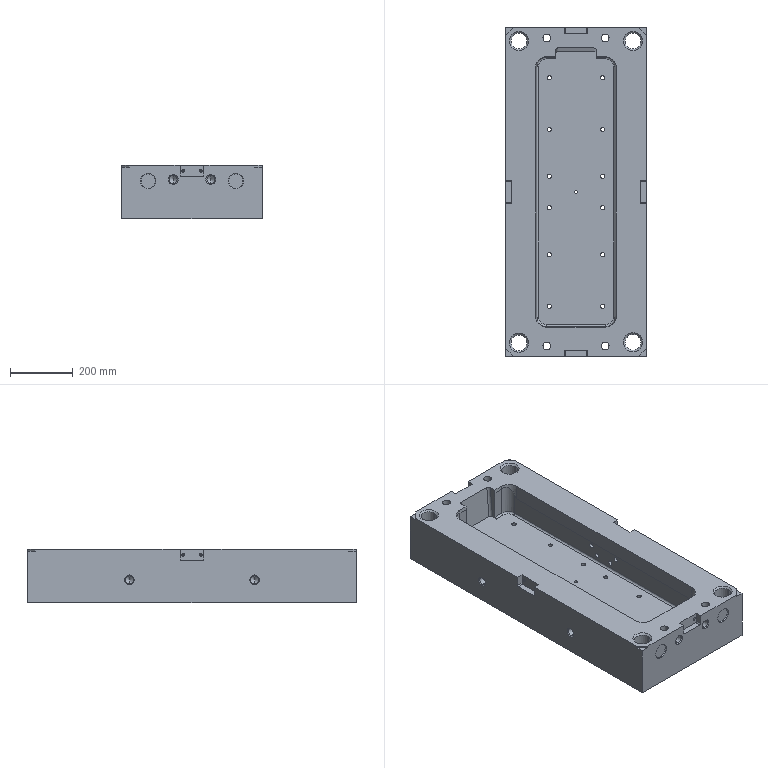Part | STEP file | 4-20.sldasm-Part-380 | 1 solid | 381 faces | box 450 x 1050 x 170 mm | volume 53576384 mm3 | cylinder 185 | plane 112 | cone 80 | torus 4 | commonest cylinder face diameters 13.492 x24 20.638 x24 25.4 x24 8.237 x16 10 x16 8 x8